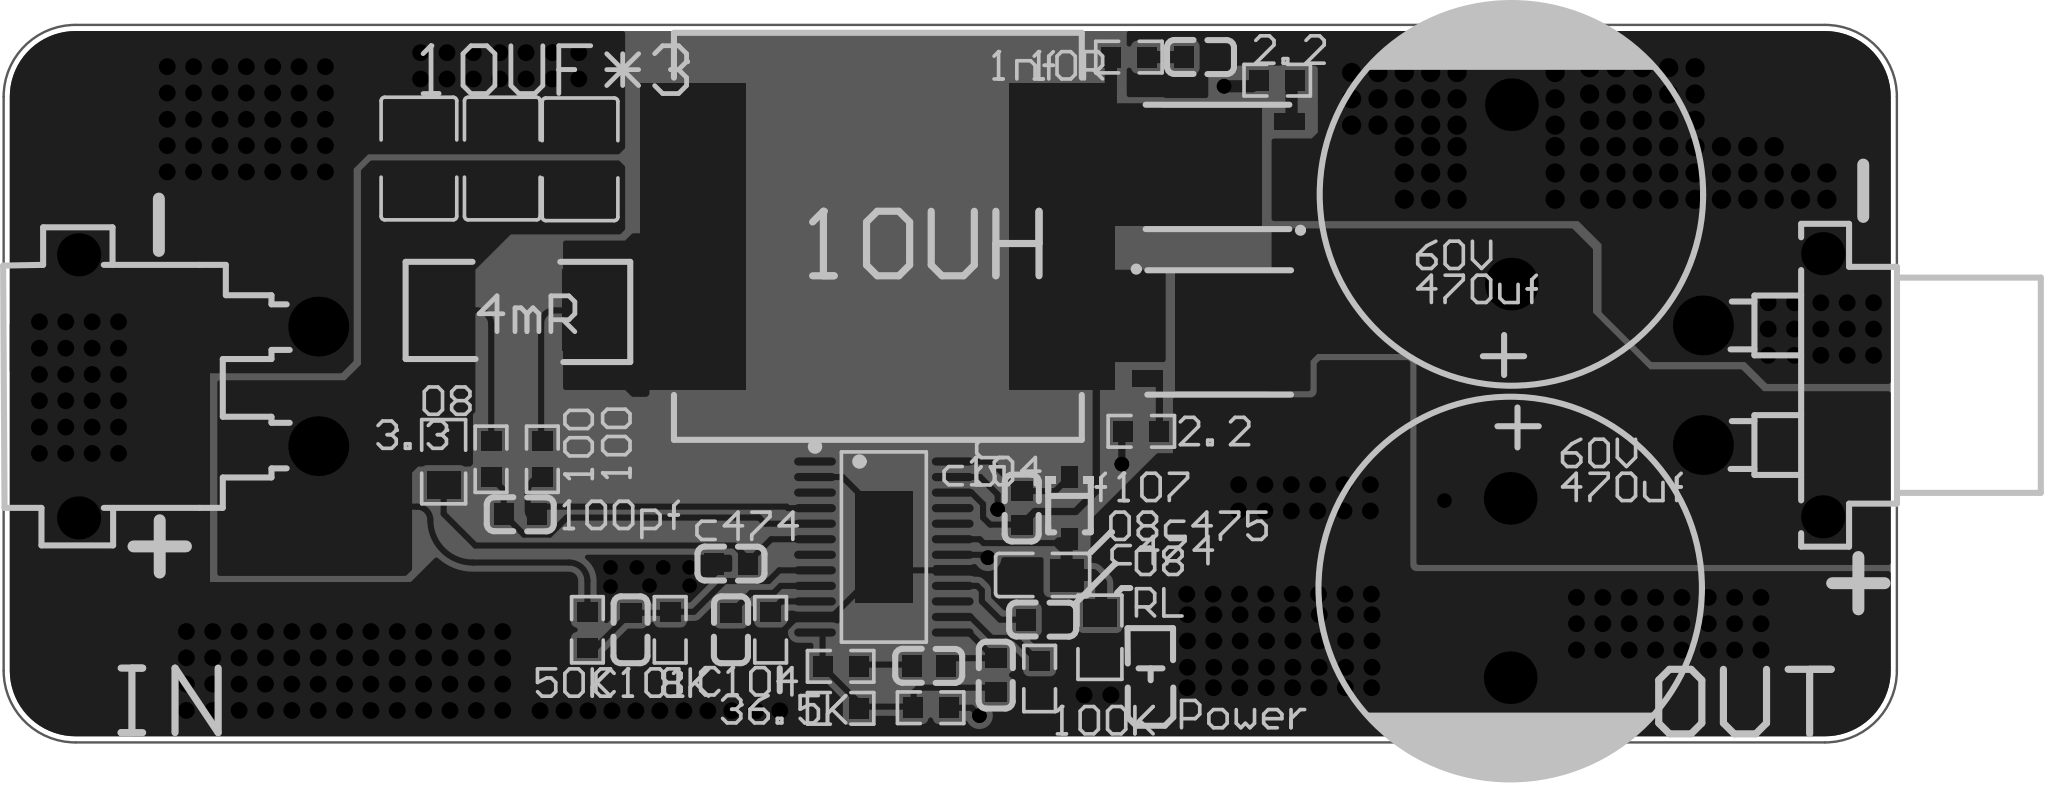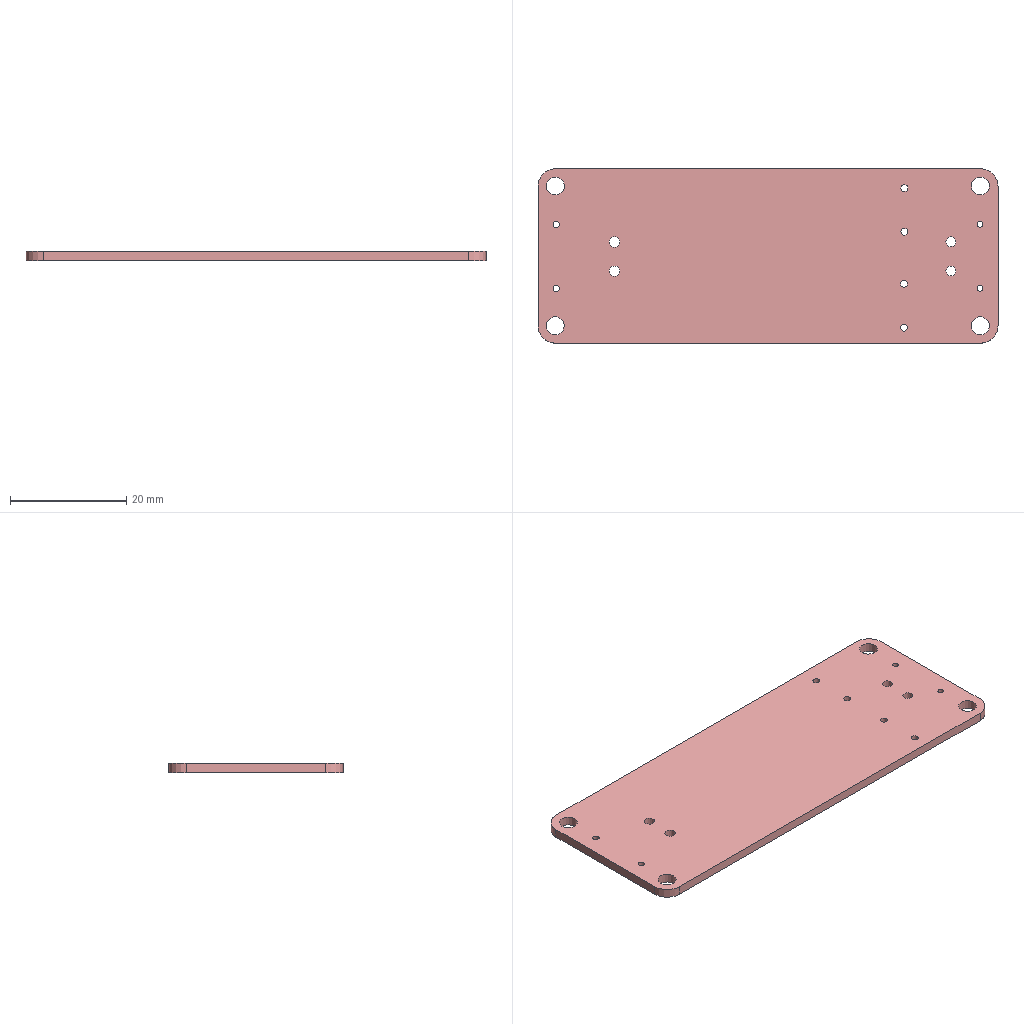Circuit board layout | Altium Designer | box 79 x 30 x 1.6 mm
Layer stack:
# Altium Designer layer stack of  (unit mm; dielectric type: 0 none, 1 core, 2 prepreg, 3 surface material)
index,name,kind,layer,copper_thickness_mm,dielectric_type,dielectric_thickness_mm,dielectric_material,dielectric_constant
0,Top Paste Mask Layer,other,,,,,,
1,Top Silkscreen Layer,other,,,,,,
2,Top Solder Mask Layer,dielectric,,,3,0.01,,3.3
3,Top Layer,copper,Top Layer,0.035,,,,
4,Dielectric1,dielectric,,,3,1.51,FR4,4.5
5,Bottom Layer,copper,Bottom Layer,0.035,,,,
6,Bottom Solder Mask Layer,dielectric,,,3,0.01,,3.3
7,Bottom Silkscreen Layer,other,,,,,,
8,Bottom Paste Mask Layer,other,,,,,,
# drill layer pairs: low layer,high layer
drill_pair,Top Layer,Bottom Layer
Part placement:
Designator,Comment,Layer,Footprint,Center-X(mm),Center-Y(mm),Rotation
R1,50K,TopLayer,R0603,104.394,83.244,90
R2,8K,TopLayer,R0603,107.848,83.244,90
C1,100pF,TopLayer,C0603,106.197,83.251,90
C2,470nF,TopLayer,C0603,110.393,86.009,0
C3,100nF,TopLayer,C0603,110.388,83.251,90
R4,36.5K,TopLayer,R0603,112.039,83.244,90
R6,4mΩ,TopLayer,RES-SMD_L6.4-W3.2-1,101.496,96.596,0
U2,10uH,TopLayer,IND-SMD_L17.0-W17.0_YSPIA1770-100M,116.515,99.695,0
C5,300pF,TopLayer,C0603,121.437,81.356,90
C6,34nF,TopLayer,C0603,118.643,81.733,0
R7,40.53K,TopLayer,R0603,114.96,81.715,0
R8,1.6K,TopLayer,R0603,114.96,79.959,0
R9,30K,TopLayer,R0603,118.716,79.984,0
R13,10K,TopLayer,R0603,127.508,91.542,0
R11,100K,TopLayer,R0603,123.265,81.205,90
C7,470nF,TopLayer,C0603,123.397,83.668,0
C8,4.7uf,TopLayer,C0805,123.39,85.534,180
C9,100nF,TopLayer,C0603,122.521,88.341,90
U3,FR107WS,TopLayer,SOD-323_L1.6-W1.3-LS2.7-RD,124.511,88.334,270
Q1,CSD18540Q5B,TopLayer,VSON-CLIP-8_L5.0-W6.0-P1.27-BL,130.757,95.675,270
Q2,CSD18540Q5B,TopLayer,VSON-CLIP-8_L5.0-W6.0-P1.27-BL,130.687,102.596,90
C10,100pf,TopLayer,C0603,101.6,88.07,0
R14,100,TopLayer,R0603,100.372,90.373,90
R15,100,TopLayer,R0603,102.514,90.373,90
C11,10uF,TopLayer,C1210,100.842,102.946,270
C12,10uF,TopLayer,C1210,97.364,102.946,270
C13,10uF,TopLayer,C1210,104.088,102.914,270
R12,2.2,TopLayer,R0603,133.178,106.223,0
R5,3.3,TopLayer,R0805_NEW,98.396,90.272,90
CN3,XT30PW-M,TopLayer,CONN-TH_XT30PW-M,88.163,93.421,270
U4,XT30PW-F,TopLayer,CONN-TH_XT30PW-F-1,153.441,93.468,90
U5,LM5122ZAPWPR,TopLayer,HTSSOP-24_L7.8-W4.4-P0.65-LS6.4-BL-EP-3,116.764,86.704,270
C20,470uF,TopLayer,CAP-TH_BD16.0-P7.50-D1.2-FD,142.9,84.989,270
R16,10K,TopLayer,R0603,126.991,107.188,0
C18,100nF,TopLayer,C0603,129.984,107.188,0
C21,470uF,TopLayer,CAP-TH_BD16.0-P7.50-D1.2-FD,142.951,101.448,90
LED1,,TopLayer,LED_0805,127.892,81.332,90
R17,10K,TopLayer,R0805,125.781,82.931,90
Pad and via stacks:
# Altium Designer via and pad stacks of  (unit mm). Each distinct definition once, with the count of objects using it.
# via: kind,start_layer,end_layer,hole_mm,diameter_mm,mode(0 simple;1 top-mid-bottom;2 full stack),diameter_per_layer,count,example_net
# pad: kind,layer,hole_mm,hole_type(0 round;1 square;2 slot),plating,top_size,top_shape(1 round;2 rect;3 octagon;9 rounded rect),mid_size,bottom_size,mode,footprint,size_per_layer,count,example
pad,Top Layer,0,0,plated,5x3,1,5x3,5x3,0,,,4,1
pad,Top Layer,0,0,plated,0.8065x0.864,2,0.8065x0.864,0.8065x0.864,0,R0603,,24,R1.2
pad,Top Layer,0,0,plated,0.8x0.9,2,0.8x0.9,0.8x0.9,0,C0603,,18,C1.2
pad,Top Layer,0,0,plated,2.5x3.4,2,2.5x3.4,2.5x3.4,0,RES-SMD_L6.4-W3.2-1,,2,R6.2
pad,Top Layer,0,0,plated,4.4x12.8,2,4.4x12.8,4.4x12.8,0,IND-SMD_L17.0-W17.0_YSPIA1770-100M,,2,U2.2
pad,Top Layer,0,0,plated,1.41x1.35,2,1.41x1.35,1.41x1.35,0,C0805,,2,C8.2
pad,Top Layer,0,0,plated,0.9x0.7,2,0.9x0.7,0.9x0.7,0,SOD-323_L1.6-W1.3-LS2.7-RD,,2,U3.2
pad,Top Layer,0,0,plated,0.7x1.27,2,0.7x1.27,0.7x1.27,0,VSON-CLIP-8_L5.0-W6.0-P1.27-BL,,8,Q1.1
pad,Top Layer,0,0,plated,4.9x4.5,2,4.9x4.5,4.9x4.5,0,VSON-CLIP-8_L5.0-W6.0-P1.27-BL,,2,Q1.8
pad,Top Layer,0,0,plated,0.7x1,2,0.7x1,0.7x1,0,VSON-CLIP-8_L5.0-W6.0-P1.27-BL,,8,Q1.8
pad,Top Layer,0,0,plated,1.635x2.7,2,1.635x2.7,1.635x2.7,0,C1210,,6,C11.2
pad,Top Layer,0,0,plated,1.133x1.377,2,1.133x1.377,1.133x1.377,0,R0805_NEW,,2,R5.2
pad,Top Layer,0,0,plated,4.68x2.4,2,4.68x2.4,4.68x2.4,0,HTSSOP-24_L7.8-W4.4-P0.65-LS6.4-BL-EP-3,,1,U5.25
pad,Top Layer,0,0,plated,0.343x1.746,1,0.343x1.746,0.343x1.746,0,HTSSOP-24_L7.8-W4.4-P0.65-LS6.4-BL-EP-3,,24,U5.13
pad,Top Layer,0,0,plated,1x1.25,2,1x1.25,1x1.25,0,LED_0805,,2,LED1.2
pad,Top Layer,0,0,plated,1.133x1.377,2,1.133x1.377,1.133x1.377,0,R0805,,2,R17.2
pad,Multi-Layer,1.8,0,plated,2.5x2.5,1,2.5x2.5,2.5x2.5,0,CONN-TH_XT30PW-M,,2,CN3.1
pad,Multi-Layer,1.1,0,plated,1.8x1.8,1,1.8x1.8,1.8x1.8,0,CONN-TH_XT30PW-M,,2,CN3.3
pad,Multi-Layer,1,0,plated,1.8x1.8,1,1.8x1.8,1.8x1.8,0,CONN-TH_XT30PW-F-1,,2,U4.4
pad,Multi-Layer,1.7,0,plated,2.5x2.5,1,2.5x2.5,2.5x2.5,0,CONN-TH_XT30PW-F-1,,2,U4.2
pad,Multi-Layer,1.2,0,plated,2.2x2.2,1,2.2x2.2,2.2x2.2,0,CAP-TH_BD16.0-P7.50-D1.2-FD,,4,C20.2
via,Top Layer,Bottom Layer,0.3048,0.61,0,,13,$1N3140
via,Top Layer,Bottom Layer,0.3988,0.8,0,,73,AGND
via,Top Layer,Bottom Layer,0.3505,0.7,0,,229,AGND
Copper pours:
name,layer,net,type(0 solid;1 hatched;2 none)
Top Layer-AGND,Top Layer,AGND,0
Top Layer-VIN,Top Layer,VIN,0
Top Layer-$1N3575,Top Layer,$1N3575,0
Top Layer-$1N3000,Top Layer,$1N3000,0
Top Layer-$1N3000 1,Top Layer,$1N3000,0
Top Layer-AGND 1,Top Layer,AGND,0
Top Layer-VOUT,Top Layer,VOUT,0
Top Layer-AGND 2,Top Layer,AGND,0
Bottom Layer-AGND,Bottom Layer,AGND,0
Design rules, without the lines most boards share:
# Altium Designer design rules of  (exported by Altium Designer, unit mm)
# columns: name | kind | enabled | priority | scope1 | scope2 | descriptor | typed fields (field=value)
Clearance | 0 | disabled | 4 | All | All | Clearance Constraint (Gap=5.984mil) (Disabled)(All),(All) | gap=0.152
BoardOutlineClearance | 63 | disabled | 4 | All | All | Board Clearance Constraint (Gap=0mil) (Disabled)(All) |
Copper_copperRegion2 | 0 | disabled | 5 | All | All | Clearance Constraint (Gap=5.984mil) (Disabled)(All),(All) | gap=0.152
Copper_copperRegion2_1 | 63 | disabled | 5 | All | All | Board Clearance Constraint (Gap=0mil) (Disabled)(All) |
copperThickness1oz | 0 | enabled | 6 | All | All | Clearance Constraint (Gap=5.984mil) (All),(All) | gap=0.152
copperThickness1oz_1 | 63 | enabled | 6 | All | All | Board Clearance Constraint (Gap=0mil) (All) |
otherClearance | 52 | enabled | 1 | All | All | Hole To Hole Clearance (Gap=11.8mil) (All),(All) | gap=0.2997
PolygonConnect | 20 | disabled | 1 | All | All | Polygon Connect Rule(Direct Connect )(Conductor Width=10mil) (Relief Angle=90 Angle) (Entries=4) (Air Gap Width=10mil) (Disabled)(All),(All) | connect_style(0=relief,1=direct,2=none)=1 relief_conductor_width=0.254 relief_entries=4
copperRegion2 | 20 | disabled | 2 | All | All | Polygon Connect Rule(Relief Connect )(Conductor Width=10mil) (Relief Angle=90 Angle) (Entries=4) (Air Gap Width=10mil) (Disabled)(All),(All) | connect_style(0=relief,1=direct,2=none)=0 relief_conductor_width=0.254 relief_entries=4
copperRegion | 20 | enabled | 3 | All | All | Polygon Connect Rule(Relief Connect )(Conductor Width=10mil) (Relief Angle=90 Angle) (Entries=4) (Air Gap Width=10mil) (All),(All) | connect_style(0=relief,1=direct,2=none)=0 relief_conductor_width=0.254 relief_entries=4
solderMaskExpansion | 13 | enabled | 2 | All | All | Solder Mask Expansion (Expansion =2.008mil) (All) | expansion=0.051